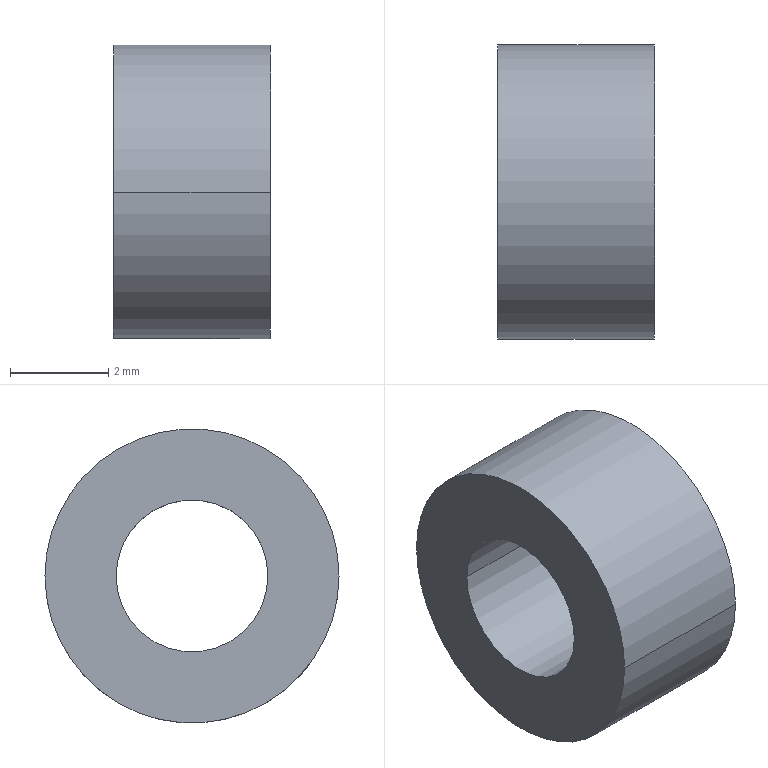Part | SolidWorks | features BaseBody 1 | 1 solid | 6 faces | box 3.205 x 6 x 6.003 mm | volume 66.325 mm3 | cylinder 4 | plane 2 | commonest cylinder face diameters 3.1 x2 6 x2
STEP:
#1=CARTESIAN_POINT('',(-257.65,-8.991,-83.66));
#2=VERTEX_POINT('',#1);
#3=CARTESIAN_POINT('',(-257.65,-5.891,-83.659));
#4=VERTEX_POINT('',#3);
#5=CARTESIAN_POINT('',(-257.65,-7.441,-83.659));
#6=DIRECTION('',(1.,0.00003864,-0.0008339));
#7=DIRECTION('',(0.00003827,-1.,-0.0004455));
#8=AXIS2_PLACEMENT_3D('',#5,#6,#7);
#9=CIRCLE('',#8,1.55);
#10=EDGE_CURVE('',#2,#4,#9,.T.);
#11=ORIENTED_EDGE('',*,*,#10,.F.);
#12=CARTESIAN_POINT('',(-257.65,-7.441,-83.659));
#13=DIRECTION('',(1.,0.00003864,-0.0008339));
#14=DIRECTION('',(-0.00003827,1.,0.0004455));
#15=AXIS2_PLACEMENT_3D('',#12,#13,#14);
#16=CIRCLE('',#15,1.55);
#17=EDGE_CURVE('',#4,#2,#16,.T.);
#18=ORIENTED_EDGE('',*,*,#17,.F.);
#19=EDGE_LOOP('',(#11,#18));
#20=FACE_BOUND('',#19,.T.);
#21=CARTESIAN_POINT('',(-257.65,-10.441,-83.661));
#22=VERTEX_POINT('',#21);
#23=CARTESIAN_POINT('',(-257.65,-4.441,-83.658));
#24=VERTEX_POINT('',#23);
#25=CARTESIAN_POINT('',(-257.65,-7.441,-83.659));
#26=DIRECTION('',(-1.,-0.00003864,0.0008339));
#27=DIRECTION('',(0.00003827,-1.,-0.0004455));
#28=AXIS2_PLACEMENT_3D('',#25,#26,#27);
#29=CIRCLE('',#28,3.);
#30=EDGE_CURVE('',#22,#24,#29,.T.);
#31=ORIENTED_EDGE('',*,*,#30,.F.);
#32=CARTESIAN_POINT('',(-257.65,-7.441,-83.659));
#33=DIRECTION('',(-1.,-0.00003864,0.0008339));
#34=DIRECTION('',(-0.00003827,1.,0.0004455));
#35=AXIS2_PLACEMENT_3D('',#32,#33,#34);
#36=CIRCLE('',#35,3.);
#37=EDGE_CURVE('',#24,#22,#36,.T.);
#38=ORIENTED_EDGE('',*,*,#37,.F.);
#39=EDGE_LOOP('',(#31,#38));
#40=FACE_OUTER_BOUND('',#39,.T.);
#41=CARTESIAN_POINT('',(-257.65,-7.441,-83.659));
#42=DIRECTION('',(-1.,-0.00003864,0.0008339));
#43=DIRECTION('',(-0.00003864,1.,0.));
#44=AXIS2_PLACEMENT_3D('',#41,#42,#43);
#45=PLANE('',#44);
#46=ADVANCED_FACE('',(#20,#40),#45,.F.);
#47=CARTESIAN_POINT('',(-260.85,-10.441,-83.658));
#48=VERTEX_POINT('',#47);
#49=CARTESIAN_POINT('',(-260.85,-4.441,-83.655));
#50=VERTEX_POINT('',#49);
#51=CARTESIAN_POINT('',(-260.85,-7.441,-83.657));
#52=DIRECTION('',(1.,0.00003864,-0.0008339));
#53=DIRECTION('',(0.00003827,-1.,-0.0004455));
#54=AXIS2_PLACEMENT_3D('',#51,#52,#53);
#55=CIRCLE('',#54,3.);
#56=EDGE_CURVE('',#48,#50,#55,.T.);
#57=ORIENTED_EDGE('',*,*,#56,.T.);
#58=CARTESIAN_POINT('',(-257.65,-4.441,-83.658));
#59=DIRECTION('',(-1.,-0.00003864,0.0008339));
#60=VECTOR('',#59,1000.);
#61=LINE('',#58,#60);
#62=EDGE_CURVE('',#24,#50,#61,.T.);
#63=ORIENTED_EDGE('',*,*,#62,.F.);
#64=ORIENTED_EDGE('',*,*,#37,.T.);
#65=CARTESIAN_POINT('',(-257.65,-10.441,-83.661));
#66=DIRECTION('',(-1.,-0.00003864,0.0008339));
#67=VECTOR('',#66,1000.);
#68=LINE('',#65,#67);
#69=EDGE_CURVE('',#22,#48,#68,.T.);
#70=ORIENTED_EDGE('',*,*,#69,.T.);
#71=EDGE_LOOP('',(#57,#63,#64,#70));
#72=FACE_OUTER_BOUND('',#71,.T.);
#73=CARTESIAN_POINT('',(-260.85,-7.441,-83.657));
#74=DIRECTION('',(1.,0.00003864,-0.0008339));
#75=DIRECTION('',(-0.00003827,1.,0.0004455));
#76=AXIS2_PLACEMENT_3D('',#73,#74,#75);
#77=CYLINDRICAL_SURFACE('',#76,3.);
#78=ADVANCED_FACE('',(#72),#77,.T.);
#79=ORIENTED_EDGE('',*,*,#69,.F.);
#80=ORIENTED_EDGE('',*,*,#30,.T.);
#81=ORIENTED_EDGE('',*,*,#62,.T.);
#82=CARTESIAN_POINT('',(-260.85,-7.441,-83.657));
#83=DIRECTION('',(1.,0.00003864,-0.0008339));
#84=DIRECTION('',(-0.00003827,1.,0.0004455));
#85=AXIS2_PLACEMENT_3D('',#82,#83,#84);
#86=CIRCLE('',#85,3.);
#87=EDGE_CURVE('',#50,#48,#86,.T.);
#88=ORIENTED_EDGE('',*,*,#87,.T.);
#89=EDGE_LOOP('',(#79,#80,#81,#88));
#90=FACE_OUTER_BOUND('',#89,.T.);
#91=CARTESIAN_POINT('',(-260.85,-7.441,-83.657));
#92=DIRECTION('',(1.,0.00003864,-0.0008339));
#93=DIRECTION('',(-0.00003827,1.,0.0004455));
#94=AXIS2_PLACEMENT_3D('',#91,#92,#93);
#95=CYLINDRICAL_SURFACE('',#94,3.);
#96=ADVANCED_FACE('',(#90),#95,.T.);
#97=CARTESIAN_POINT('',(-260.85,-5.891,-83.656));
#98=VERTEX_POINT('',#97);
#99=CARTESIAN_POINT('',(-260.85,-8.991,-83.657));
#100=VERTEX_POINT('',#99);
#101=CARTESIAN_POINT('',(-260.85,-7.441,-83.657));
#102=DIRECTION('',(-1.,-0.00003864,0.0008339));
#103=DIRECTION('',(-0.00003827,1.,0.0004455));
#104=AXIS2_PLACEMENT_3D('',#101,#102,#103);
#105=CIRCLE('',#104,1.55);
#106=EDGE_CURVE('',#98,#100,#105,.T.);
#107=ORIENTED_EDGE('',*,*,#106,.F.);
#108=CARTESIAN_POINT('',(-260.85,-7.441,-83.657));
#109=DIRECTION('',(-1.,-0.00003864,0.0008339));
#110=DIRECTION('',(0.00003827,-1.,-0.0004455));
#111=AXIS2_PLACEMENT_3D('',#108,#109,#110);
#112=CIRCLE('',#111,1.55);
#113=EDGE_CURVE('',#100,#98,#112,.T.);
#114=ORIENTED_EDGE('',*,*,#113,.F.);
#115=EDGE_LOOP('',(#107,#114));
#116=FACE_BOUND('',#115,.T.);
#117=ORIENTED_EDGE('',*,*,#87,.F.);
#118=ORIENTED_EDGE('',*,*,#56,.F.);
#119=EDGE_LOOP('',(#117,#118));
#120=FACE_OUTER_BOUND('',#119,.T.);
#121=CARTESIAN_POINT('',(-260.85,-7.441,-83.657));
#122=DIRECTION('',(-1.,-0.00003864,0.0008339));
#123=DIRECTION('',(-0.00003864,1.,0.));
#124=AXIS2_PLACEMENT_3D('',#121,#122,#123);
#125=PLANE('',#124);
#126=ADVANCED_FACE('',(#116,#120),#125,.T.);
#127=ORIENTED_EDGE('',*,*,#17,.T.);
#128=CARTESIAN_POINT('',(-260.85,-8.991,-83.657));
#129=DIRECTION('',(1.,0.00003864,-0.0008339));
#130=VECTOR('',#129,1000.);
#131=LINE('',#128,#130);
#132=EDGE_CURVE('',#100,#2,#131,.T.);
#133=ORIENTED_EDGE('',*,*,#132,.F.);
#134=ORIENTED_EDGE('',*,*,#113,.T.);
#135=CARTESIAN_POINT('',(-260.85,-5.891,-83.656));
#136=DIRECTION('',(1.,0.00003864,-0.0008339));
#137=VECTOR('',#136,1000.);
#138=LINE('',#135,#137);
#139=EDGE_CURVE('',#98,#4,#138,.T.);
#140=ORIENTED_EDGE('',*,*,#139,.T.);
#141=EDGE_LOOP('',(#127,#133,#134,#140));
#142=FACE_OUTER_BOUND('',#141,.T.);
#143=CARTESIAN_POINT('',(-257.65,-7.441,-83.659));
#144=DIRECTION('',(-1.,-0.00003864,0.0008339));
#145=DIRECTION('',(0.00003827,-1.,-0.0004455));
#146=AXIS2_PLACEMENT_3D('',#143,#144,#145);
#147=CYLINDRICAL_SURFACE('',#146,1.55);
#148=ADVANCED_FACE('',(#142),#147,.F.);
#149=ORIENTED_EDGE('',*,*,#139,.F.);
#150=ORIENTED_EDGE('',*,*,#106,.T.);
#151=ORIENTED_EDGE('',*,*,#132,.T.);
#152=ORIENTED_EDGE('',*,*,#10,.T.);
#153=EDGE_LOOP('',(#149,#150,#151,#152));
#154=FACE_OUTER_BOUND('',#153,.T.);
#155=CARTESIAN_POINT('',(-257.65,-7.441,-83.659));
#156=DIRECTION('',(-1.,-0.00003864,0.0008339));
#157=DIRECTION('',(0.00003827,-1.,-0.0004455));
#158=AXIS2_PLACEMENT_3D('',#155,#156,#157);
#159=CYLINDRICAL_SURFACE('',#158,1.55);
#160=ADVANCED_FACE('',(#154),#159,.F.);
#161=CLOSED_SHELL('',(#46,#78,#96,#126,#148,#160));
#162=MANIFOLD_SOLID_BREP('',#161);
#163=CARTESIAN_POINT('',(0.,0.,0.));
#164=DIRECTION('',(0.,0.,1.));
#165=DIRECTION('',(1.,0.,0.));
#166=AXIS2_PLACEMENT_3D('',#163,#164,#165);
#167=(LENGTH_UNIT()NAMED_UNIT(*)SI_UNIT(.MILLI.,.METRE.));
#168=UNCERTAINTY_MEASURE_WITH_UNIT(LENGTH_MEASURE(0.00001),#167,'','');
#169=(NAMED_UNIT(*)PLANE_ANGLE_UNIT()SI_UNIT($,.RADIAN.));
#170=(NAMED_UNIT(*)SI_UNIT($,.STERADIAN.)SOLID_ANGLE_UNIT());
#171=(GEOMETRIC_REPRESENTATION_CONTEXT(3)GLOBAL_UNCERTAINTY_ASSIGNED_CONTEXT((#168))GLOBAL_UNIT_ASSIGNED_CONTEXT((#167,#169,#170))REPRESENTATION_CONTEXT('',''));
#172=ADVANCED_BREP_SHAPE_REPRESENTATION('',(#162,#166),#171);